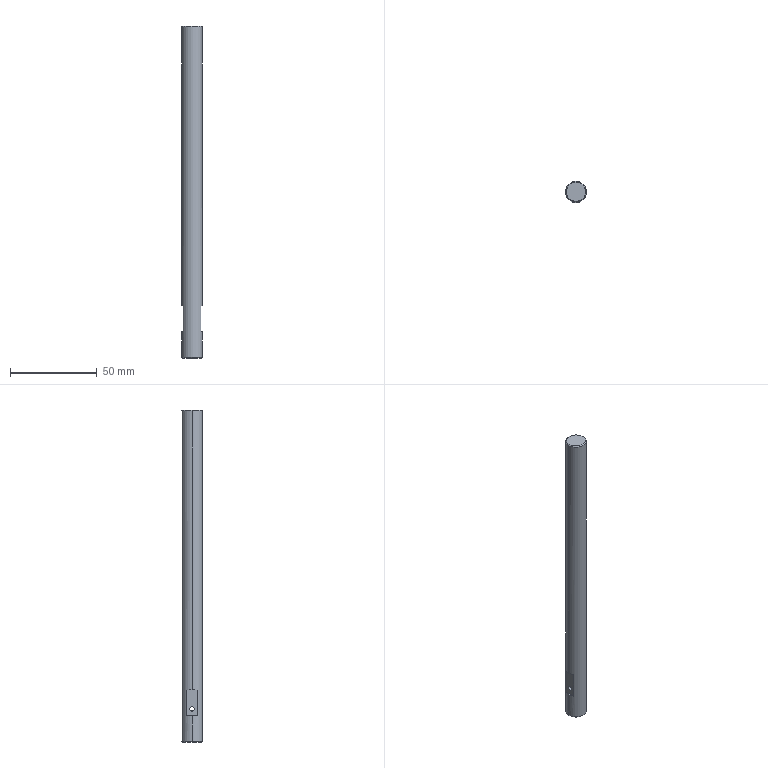Part | STEP file | 2009 Bag feed support shaft B | 1 solid | 20 faces | box 12 x 12 x 191 mm | volume 21066 mm3 | plane 8 | cylinder 6 | cone 6 | commonest cylinder face diameters 2.5 x2 5 x2 12 x2